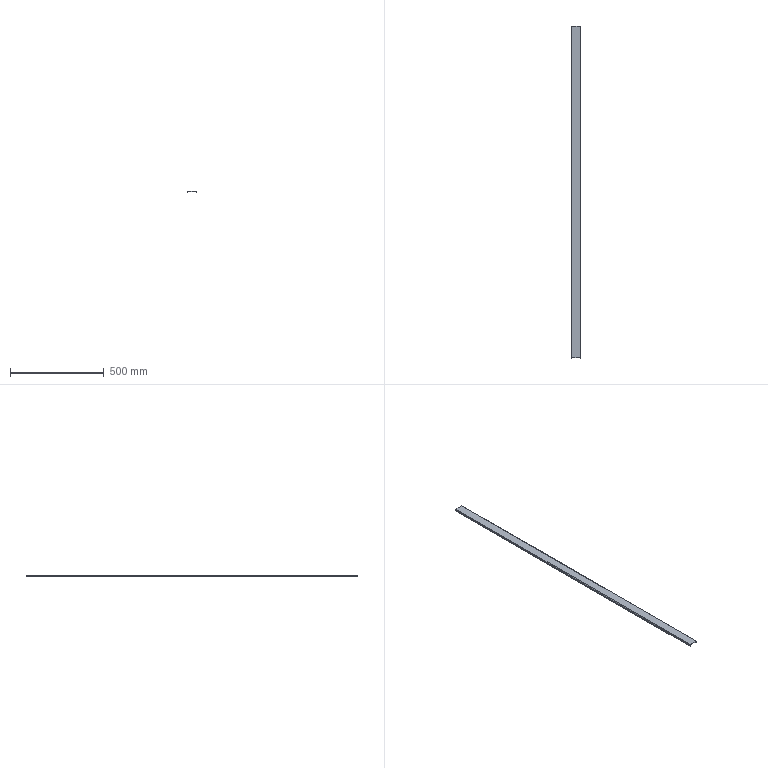Part | SolidWorks | features BaseBody 1 | 1 solid | 22 faces | box 50 x 1772 x 10 mm | volume 281263 mm3 | plane 18 | cylinder 4 | commonest cylinder face diameters 1 x2 6 x2
STEP:
#1=CARTESIAN_POINT('',(-22.5,885.9,-10.));
#2=VERTEX_POINT('',#1);
#3=CARTESIAN_POINT('',(-22.5,-885.9,-10.));
#4=VERTEX_POINT('',#3);
#5=CARTESIAN_POINT('',(-22.5,-885.9,-10.));
#6=DIRECTION('',(0.,-1.,0.));
#7=VECTOR('',#6,1000.);
#8=LINE('',#5,#7);
#9=EDGE_CURVE('',#2,#4,#8,.T.);
#10=ORIENTED_EDGE('',*,*,#9,.T.);
#11=CARTESIAN_POINT('',(-25.,-885.9,-10.));
#12=VERTEX_POINT('',#11);
#13=CARTESIAN_POINT('',(-25.,-885.9,-10.));
#14=DIRECTION('',(1.,0.,0.));
#15=VECTOR('',#14,1000.);
#16=LINE('',#13,#15);
#17=EDGE_CURVE('',#12,#4,#16,.T.);
#18=ORIENTED_EDGE('',*,*,#17,.F.);
#19=CARTESIAN_POINT('',(-25.,885.9,-10.));
#20=VERTEX_POINT('',#19);
#21=CARTESIAN_POINT('',(-25.,0.,-10.));
#22=DIRECTION('',(0.,-1.,0.));
#23=VECTOR('',#22,1000.);
#24=LINE('',#21,#23);
#25=EDGE_CURVE('',#20,#12,#24,.T.);
#26=ORIENTED_EDGE('',*,*,#25,.F.);
#27=CARTESIAN_POINT('',(-25.,885.9,-10.));
#28=DIRECTION('',(1.,0.,0.));
#29=VECTOR('',#28,1000.);
#30=LINE('',#27,#29);
#31=EDGE_CURVE('',#20,#2,#30,.T.);
#32=ORIENTED_EDGE('',*,*,#31,.T.);
#33=EDGE_LOOP('',(#10,#18,#26,#32));
#34=FACE_OUTER_BOUND('',#33,.T.);
#35=CARTESIAN_POINT('',(-25.,-885.9,-10.));
#36=DIRECTION('',(0.,0.,1.));
#37=DIRECTION('',(1.,0.,0.));
#38=AXIS2_PLACEMENT_3D('',#35,#36,#37);
#39=PLANE('',#38);
#40=ADVANCED_FACE('',(#34),#39,.F.);
#41=CARTESIAN_POINT('',(-22.5,885.9,-3.));
#42=VERTEX_POINT('',#41);
#43=CARTESIAN_POINT('',(-22.5,885.9,-10.));
#44=DIRECTION('',(0.,0.,-1.));
#45=VECTOR('',#44,1000.);
#46=LINE('',#43,#45);
#47=EDGE_CURVE('',#42,#2,#46,.T.);
#48=ORIENTED_EDGE('',*,*,#47,.F.);
#49=CARTESIAN_POINT('',(-22.5,-885.9,-3.));
#50=VERTEX_POINT('',#49);
#51=CARTESIAN_POINT('',(-22.5,-885.9,-3.));
#52=DIRECTION('',(0.,1.,0.));
#53=VECTOR('',#52,1000.);
#54=LINE('',#51,#53);
#55=EDGE_CURVE('',#50,#42,#54,.T.);
#56=ORIENTED_EDGE('',*,*,#55,.F.);
#57=CARTESIAN_POINT('',(-22.5,-885.9,-2.5));
#58=DIRECTION('',(0.,0.,1.));
#59=VECTOR('',#58,1000.);
#60=LINE('',#57,#59);
#61=EDGE_CURVE('',#4,#50,#60,.T.);
#62=ORIENTED_EDGE('',*,*,#61,.F.);
#63=ORIENTED_EDGE('',*,*,#9,.F.);
#64=EDGE_LOOP('',(#48,#56,#62,#63));
#65=FACE_OUTER_BOUND('',#64,.T.);
#66=CARTESIAN_POINT('',(-22.5,0.,0.));
#67=DIRECTION('',(1.,0.,0.));
#68=DIRECTION('',(0.,0.,-1.));
#69=AXIS2_PLACEMENT_3D('',#66,#67,#68);
#70=PLANE('',#69);
#71=ADVANCED_FACE('',(#65),#70,.T.);
#72=CARTESIAN_POINT('',(-25.,885.9,-3.));
#73=VERTEX_POINT('',#72);
#74=CARTESIAN_POINT('',(-25.,-885.9,-3.));
#75=VERTEX_POINT('',#74);
#76=CARTESIAN_POINT('',(-25.,-885.9,-3.));
#77=DIRECTION('',(0.,-1.,0.));
#78=VECTOR('',#77,1000.);
#79=LINE('',#76,#78);
#80=EDGE_CURVE('',#73,#75,#79,.T.);
#81=ORIENTED_EDGE('',*,*,#80,.F.);
#82=CARTESIAN_POINT('',(-25.,885.9,0.));
#83=DIRECTION('',(0.,0.,-1.));
#84=VECTOR('',#83,1000.);
#85=LINE('',#82,#84);
#86=EDGE_CURVE('',#73,#20,#85,.T.);
#87=ORIENTED_EDGE('',*,*,#86,.T.);
#88=ORIENTED_EDGE('',*,*,#25,.T.);
#89=CARTESIAN_POINT('',(-25.,-885.9,0.));
#90=DIRECTION('',(0.,0.,1.));
#91=VECTOR('',#90,1000.);
#92=LINE('',#89,#91);
#93=EDGE_CURVE('',#12,#75,#92,.T.);
#94=ORIENTED_EDGE('',*,*,#93,.T.);
#95=EDGE_LOOP('',(#81,#87,#88,#94));
#96=FACE_OUTER_BOUND('',#95,.T.);
#97=CARTESIAN_POINT('',(-25.,0.,0.));
#98=DIRECTION('',(1.,0.,0.));
#99=DIRECTION('',(0.,0.,-1.));
#100=AXIS2_PLACEMENT_3D('',#97,#98,#99);
#101=PLANE('',#100);
#102=ADVANCED_FACE('',(#96),#101,.F.);
#103=CARTESIAN_POINT('',(-25.,-885.9,-3.));
#104=DIRECTION('',(-1.,0.,0.));
#105=VECTOR('',#104,1000.);
#106=LINE('',#103,#105);
#107=EDGE_CURVE('',#50,#75,#106,.T.);
#108=ORIENTED_EDGE('',*,*,#107,.T.);
#109=ORIENTED_EDGE('',*,*,#93,.F.);
#110=ORIENTED_EDGE('',*,*,#17,.T.);
#111=ORIENTED_EDGE('',*,*,#61,.T.);
#112=EDGE_LOOP('',(#108,#109,#110,#111));
#113=FACE_OUTER_BOUND('',#112,.T.);
#114=CARTESIAN_POINT('',(-25.,-885.9,-2.5));
#115=DIRECTION('',(0.,1.,0.));
#116=DIRECTION('',(1.,0.,0.));
#117=AXIS2_PLACEMENT_3D('',#114,#115,#116);
#118=PLANE('',#117);
#119=ADVANCED_FACE('',(#113),#118,.F.);
#120=CARTESIAN_POINT('',(-22.5,885.9,-3.));
#121=DIRECTION('',(-1.,0.,0.));
#122=VECTOR('',#121,1000.);
#123=LINE('',#120,#122);
#124=EDGE_CURVE('',#42,#73,#123,.T.);
#125=ORIENTED_EDGE('',*,*,#124,.F.);
#126=ORIENTED_EDGE('',*,*,#47,.T.);
#127=ORIENTED_EDGE('',*,*,#31,.F.);
#128=ORIENTED_EDGE('',*,*,#86,.F.);
#129=EDGE_LOOP('',(#125,#126,#127,#128));
#130=FACE_OUTER_BOUND('',#129,.T.);
#131=CARTESIAN_POINT('',(-25.,885.9,-10.));
#132=DIRECTION('',(0.,-1.,0.));
#133=DIRECTION('',(0.,0.,-1.));
#134=AXIS2_PLACEMENT_3D('',#131,#132,#133);
#135=PLANE('',#134);
#136=ADVANCED_FACE('',(#130),#135,.F.);
#137=CARTESIAN_POINT('',(-22.,885.9,-2.5));
#138=VERTEX_POINT('',#137);
#139=CARTESIAN_POINT('',(-22.,-885.9,-2.5));
#140=VERTEX_POINT('',#139);
#141=CARTESIAN_POINT('',(-22.,885.9,-2.5));
#142=DIRECTION('',(0.,-1.,0.));
#143=VECTOR('',#142,1000.);
#144=LINE('',#141,#143);
#145=EDGE_CURVE('',#138,#140,#144,.T.);
#146=ORIENTED_EDGE('',*,*,#145,.T.);
#147=CARTESIAN_POINT('',(-22.,-885.9,-3.));
#148=DIRECTION('',(0.,-1.,0.));
#149=DIRECTION('',(0.,0.,1.));
#150=AXIS2_PLACEMENT_3D('',#147,#148,#149);
#151=CIRCLE('',#150,0.5);
#152=EDGE_CURVE('',#140,#50,#151,.T.);
#153=ORIENTED_EDGE('',*,*,#152,.T.);
#154=ORIENTED_EDGE('',*,*,#55,.T.);
#155=CARTESIAN_POINT('',(-22.,885.9,-3.));
#156=DIRECTION('',(0.,1.,0.));
#157=DIRECTION('',(0.,0.,1.));
#158=AXIS2_PLACEMENT_3D('',#155,#156,#157);
#159=CIRCLE('',#158,0.5);
#160=EDGE_CURVE('',#42,#138,#159,.T.);
#161=ORIENTED_EDGE('',*,*,#160,.T.);
#162=EDGE_LOOP('',(#146,#153,#154,#161));
#163=FACE_OUTER_BOUND('',#162,.T.);
#164=CARTESIAN_POINT('',(-22.,885.9,-3.));
#165=DIRECTION('',(0.,1.,0.));
#166=DIRECTION('',(-1.,0.,0.));
#167=AXIS2_PLACEMENT_3D('',#164,#165,#166);
#168=CYLINDRICAL_SURFACE('',#167,0.5);
#169=ADVANCED_FACE('',(#163),#168,.F.);
#170=CARTESIAN_POINT('',(-22.,885.9,0.));
#171=VERTEX_POINT('',#170);
#172=CARTESIAN_POINT('',(-22.,-885.9,0.));
#173=VERTEX_POINT('',#172);
#174=CARTESIAN_POINT('',(-22.,885.9,0.));
#175=DIRECTION('',(0.,-1.,0.));
#176=VECTOR('',#175,1000.);
#177=LINE('',#174,#176);
#178=EDGE_CURVE('',#171,#173,#177,.T.);
#179=ORIENTED_EDGE('',*,*,#178,.F.);
#180=CARTESIAN_POINT('',(-22.,885.9,-3.));
#181=DIRECTION('',(0.,1.,0.));
#182=DIRECTION('',(0.,0.,1.));
#183=AXIS2_PLACEMENT_3D('',#180,#181,#182);
#184=CIRCLE('',#183,3.);
#185=EDGE_CURVE('',#73,#171,#184,.T.);
#186=ORIENTED_EDGE('',*,*,#185,.F.);
#187=ORIENTED_EDGE('',*,*,#80,.T.);
#188=CARTESIAN_POINT('',(-22.,-885.9,-3.));
#189=DIRECTION('',(0.,-1.,0.));
#190=DIRECTION('',(0.,0.,1.));
#191=AXIS2_PLACEMENT_3D('',#188,#189,#190);
#192=CIRCLE('',#191,3.);
#193=EDGE_CURVE('',#173,#75,#192,.T.);
#194=ORIENTED_EDGE('',*,*,#193,.F.);
#195=EDGE_LOOP('',(#179,#186,#187,#194));
#196=FACE_OUTER_BOUND('',#195,.T.);
#197=CARTESIAN_POINT('',(-22.,885.9,-3.));
#198=DIRECTION('',(0.,1.,0.));
#199=DIRECTION('',(-1.,0.,0.));
#200=AXIS2_PLACEMENT_3D('',#197,#198,#199);
#201=CYLINDRICAL_SURFACE('',#200,3.);
#202=ADVANCED_FACE('',(#196),#201,.T.);
#203=ORIENTED_EDGE('',*,*,#160,.F.);
#204=ORIENTED_EDGE('',*,*,#124,.T.);
#205=ORIENTED_EDGE('',*,*,#185,.T.);
#206=CARTESIAN_POINT('',(-22.,885.9,-2.5));
#207=DIRECTION('',(0.,0.,1.));
#208=VECTOR('',#207,1000.);
#209=LINE('',#206,#208);
#210=EDGE_CURVE('',#138,#171,#209,.T.);
#211=ORIENTED_EDGE('',*,*,#210,.F.);
#212=EDGE_LOOP('',(#203,#204,#205,#211));
#213=FACE_OUTER_BOUND('',#212,.T.);
#214=CARTESIAN_POINT('',(-22.,885.9,-3.));
#215=DIRECTION('',(0.,-1.,0.));
#216=DIRECTION('',(0.,0.,-1.));
#217=AXIS2_PLACEMENT_3D('',#214,#215,#216);
#218=PLANE('',#217);
#219=ADVANCED_FACE('',(#213),#218,.F.);
#220=ORIENTED_EDGE('',*,*,#107,.F.);
#221=ORIENTED_EDGE('',*,*,#152,.F.);
#222=CARTESIAN_POINT('',(-22.,-885.9,-2.5));
#223=DIRECTION('',(0.,0.,1.));
#224=VECTOR('',#223,1000.);
#225=LINE('',#222,#224);
#226=EDGE_CURVE('',#140,#173,#225,.T.);
#227=ORIENTED_EDGE('',*,*,#226,.T.);
#228=ORIENTED_EDGE('',*,*,#193,.T.);
#229=EDGE_LOOP('',(#220,#221,#227,#228));
#230=FACE_OUTER_BOUND('',#229,.T.);
#231=CARTESIAN_POINT('',(-22.,-885.9,-3.));
#232=DIRECTION('',(0.,-1.,0.));
#233=DIRECTION('',(0.,0.,-1.));
#234=AXIS2_PLACEMENT_3D('',#231,#232,#233);
#235=PLANE('',#234);
#236=ADVANCED_FACE('',(#230),#235,.T.);
#237=CARTESIAN_POINT('',(22.5,-885.9,-10.));
#238=VERTEX_POINT('',#237);
#239=CARTESIAN_POINT('',(22.5,885.9,-10.));
#240=VERTEX_POINT('',#239);
#241=CARTESIAN_POINT('',(22.5,885.9,-10.));
#242=DIRECTION('',(0.,1.,0.));
#243=VECTOR('',#242,1000.);
#244=LINE('',#241,#243);
#245=EDGE_CURVE('',#238,#240,#244,.T.);
#246=ORIENTED_EDGE('',*,*,#245,.T.);
#247=CARTESIAN_POINT('',(25.,885.9,-10.));
#248=VERTEX_POINT('',#247);
#249=CARTESIAN_POINT('',(25.,885.9,-10.));
#250=DIRECTION('',(-1.,0.,0.));
#251=VECTOR('',#250,1000.);
#252=LINE('',#249,#251);
#253=EDGE_CURVE('',#248,#240,#252,.T.);
#254=ORIENTED_EDGE('',*,*,#253,.F.);
#255=CARTESIAN_POINT('',(25.,-885.9,-10.));
#256=VERTEX_POINT('',#255);
#257=CARTESIAN_POINT('',(25.,0.,-10.));
#258=DIRECTION('',(0.,1.,0.));
#259=VECTOR('',#258,1000.);
#260=LINE('',#257,#259);
#261=EDGE_CURVE('',#256,#248,#260,.T.);
#262=ORIENTED_EDGE('',*,*,#261,.F.);
#263=CARTESIAN_POINT('',(25.,-885.9,-10.));
#264=DIRECTION('',(-1.,0.,0.));
#265=VECTOR('',#264,1000.);
#266=LINE('',#263,#265);
#267=EDGE_CURVE('',#256,#238,#266,.T.);
#268=ORIENTED_EDGE('',*,*,#267,.T.);
#269=EDGE_LOOP('',(#246,#254,#262,#268));
#270=FACE_OUTER_BOUND('',#269,.T.);
#271=CARTESIAN_POINT('',(25.,885.9,-10.));
#272=DIRECTION('',(0.,0.,1.));
#273=DIRECTION('',(1.,0.,0.));
#274=AXIS2_PLACEMENT_3D('',#271,#272,#273);
#275=PLANE('',#274);
#276=ADVANCED_FACE('',(#270),#275,.F.);
#277=CARTESIAN_POINT('',(22.5,-885.9,-3.));
#278=VERTEX_POINT('',#277);
#279=CARTESIAN_POINT('',(22.5,-885.9,-10.));
#280=DIRECTION('',(0.,0.,-1.));
#281=VECTOR('',#280,1000.);
#282=LINE('',#279,#281);
#283=EDGE_CURVE('',#278,#238,#282,.T.);
#284=ORIENTED_EDGE('',*,*,#283,.F.);
#285=CARTESIAN_POINT('',(22.5,885.9,-3.));
#286=VERTEX_POINT('',#285);
#287=CARTESIAN_POINT('',(22.5,885.9,-3.));
#288=DIRECTION('',(0.,-1.,0.));
#289=VECTOR('',#288,1000.);
#290=LINE('',#287,#289);
#291=EDGE_CURVE('',#286,#278,#290,.T.);
#292=ORIENTED_EDGE('',*,*,#291,.F.);
#293=CARTESIAN_POINT('',(22.5,885.9,-2.5));
#294=DIRECTION('',(0.,0.,1.));
#295=VECTOR('',#294,1000.);
#296=LINE('',#293,#295);
#297=EDGE_CURVE('',#240,#286,#296,.T.);
#298=ORIENTED_EDGE('',*,*,#297,.F.);
#299=ORIENTED_EDGE('',*,*,#245,.F.);
#300=EDGE_LOOP('',(#284,#292,#298,#299));
#301=FACE_OUTER_BOUND('',#300,.T.);
#302=CARTESIAN_POINT('',(22.5,0.,0.));
#303=DIRECTION('',(-1.,0.,0.));
#304=DIRECTION('',(0.,0.,1.));
#305=AXIS2_PLACEMENT_3D('',#302,#303,#304);
#306=PLANE('',#305);
#307=ADVANCED_FACE('',(#301),#306,.T.);
#308=CARTESIAN_POINT('',(25.,-885.9,-3.));
#309=VERTEX_POINT('',#308);
#310=CARTESIAN_POINT('',(25.,885.9,-3.));
#311=VERTEX_POINT('',#310);
#312=CARTESIAN_POINT('',(25.,885.9,-3.));
#313=DIRECTION('',(0.,1.,0.));
#314=VECTOR('',#313,1000.);
#315=LINE('',#312,#314);
#316=EDGE_CURVE('',#309,#311,#315,.T.);
#317=ORIENTED_EDGE('',*,*,#316,.F.);
#318=CARTESIAN_POINT('',(25.,-885.9,0.));
#319=DIRECTION('',(0.,0.,-1.));
#320=VECTOR('',#319,1000.);
#321=LINE('',#318,#320);
#322=EDGE_CURVE('',#309,#256,#321,.T.);
#323=ORIENTED_EDGE('',*,*,#322,.T.);
#324=ORIENTED_EDGE('',*,*,#261,.T.);
#325=CARTESIAN_POINT('',(25.,885.9,0.));
#326=DIRECTION('',(0.,0.,1.));
#327=VECTOR('',#326,1000.);
#328=LINE('',#325,#327);
#329=EDGE_CURVE('',#248,#311,#328,.T.);
#330=ORIENTED_EDGE('',*,*,#329,.T.);
#331=EDGE_LOOP('',(#317,#323,#324,#330));
#332=FACE_OUTER_BOUND('',#331,.T.);
#333=CARTESIAN_POINT('',(25.,0.,0.));
#334=DIRECTION('',(-1.,0.,0.));
#335=DIRECTION('',(0.,0.,1.));
#336=AXIS2_PLACEMENT_3D('',#333,#334,#335);
#337=PLANE('',#336);
#338=ADVANCED_FACE('',(#332),#337,.F.);
#339=CARTESIAN_POINT('',(25.,885.9,-3.));
#340=DIRECTION('',(1.,0.,0.));
#341=VECTOR('',#340,1000.);
#342=LINE('',#339,#341);
#343=EDGE_CURVE('',#286,#311,#342,.T.);
#344=ORIENTED_EDGE('',*,*,#343,.T.);
#345=ORIENTED_EDGE('',*,*,#329,.F.);
#346=ORIENTED_EDGE('',*,*,#253,.T.);
#347=ORIENTED_EDGE('',*,*,#297,.T.);
#348=EDGE_LOOP('',(#344,#345,#346,#347));
#349=FACE_OUTER_BOUND('',#348,.T.);
#350=CARTESIAN_POINT('',(25.,885.9,-2.5));
#351=DIRECTION('',(0.,-1.,0.));
#352=DIRECTION('',(0.,0.,-1.));
#353=AXIS2_PLACEMENT_3D('',#350,#351,#352);
#354=PLANE('',#353);
#355=ADVANCED_FACE('',(#349),#354,.F.);
#356=CARTESIAN_POINT('',(22.5,-885.9,-3.));
#357=DIRECTION('',(1.,0.,0.));
#358=VECTOR('',#357,1000.);
#359=LINE('',#356,#358);
#360=EDGE_CURVE('',#278,#309,#359,.T.);
#361=ORIENTED_EDGE('',*,*,#360,.F.);
#362=ORIENTED_EDGE('',*,*,#283,.T.);
#363=ORIENTED_EDGE('',*,*,#267,.F.);
#364=ORIENTED_EDGE('',*,*,#322,.F.);
#365=EDGE_LOOP('',(#361,#362,#363,#364));
#366=FACE_OUTER_BOUND('',#365,.T.);
#367=CARTESIAN_POINT('',(25.,-885.9,-10.));
#368=DIRECTION('',(0.,1.,0.));
#369=DIRECTION('',(1.,0.,0.));
#370=AXIS2_PLACEMENT_3D('',#367,#368,#369);
#371=PLANE('',#370);
#372=ADVANCED_FACE('',(#366),#371,.F.);
#373=CARTESIAN_POINT('',(22.,-885.9,-2.5));
#374=VERTEX_POINT('',#373);
#375=CARTESIAN_POINT('',(22.,885.9,-2.5));
#376=VERTEX_POINT('',#375);
#377=CARTESIAN_POINT('',(22.,-885.9,-2.5));
#378=DIRECTION('',(0.,1.,0.));
#379=VECTOR('',#378,1000.);
#380=LINE('',#377,#379);
#381=EDGE_CURVE('',#374,#376,#380,.T.);
#382=ORIENTED_EDGE('',*,*,#381,.T.);
#383=CARTESIAN_POINT('',(22.,885.9,-3.));
#384=DIRECTION('',(0.,1.,0.));
#385=DIRECTION('',(0.,0.,-1.));
#386=AXIS2_PLACEMENT_3D('',#383,#384,#385);
#387=CIRCLE('',#386,0.5);
#388=EDGE_CURVE('',#376,#286,#387,.T.);
#389=ORIENTED_EDGE('',*,*,#388,.T.);
#390=ORIENTED_EDGE('',*,*,#291,.T.);
#391=CARTESIAN_POINT('',(22.,-885.9,-3.));
#392=DIRECTION('',(0.,-1.,0.));
#393=DIRECTION('',(0.,0.,-1.));
#394=AXIS2_PLACEMENT_3D('',#391,#392,#393);
#395=CIRCLE('',#394,0.5);
#396=EDGE_CURVE('',#278,#374,#395,.T.);
#397=ORIENTED_EDGE('',*,*,#396,.T.);
#398=EDGE_LOOP('',(#382,#389,#390,#397));
#399=FACE_OUTER_BOUND('',#398,.T.);
#400=CARTESIAN_POINT('',(22.,-885.9,-3.));
#401=DIRECTION('',(0.,-1.,0.));
#402=DIRECTION('',(1.,0.,0.));
#403=AXIS2_PLACEMENT_3D('',#400,#401,#402);
#404=CYLINDRICAL_SURFACE('',#403,0.5);
#405=ADVANCED_FACE('',(#399),#404,.F.);
#406=CARTESIAN_POINT('',(22.,-885.9,0.));
#407=VERTEX_POINT('',#406);
#408=CARTESIAN_POINT('',(22.,885.9,0.));
#409=VERTEX_POINT('',#408);
#410=CARTESIAN_POINT('',(22.,-885.9,0.));
#411=DIRECTION('',(0.,1.,0.));
#412=VECTOR('',#411,1000.);
#413=LINE('',#410,#412);
#414=EDGE_CURVE('',#407,#409,#413,.T.);
#415=ORIENTED_EDGE('',*,*,#414,.F.);
#416=CARTESIAN_POINT('',(22.,-885.9,-3.));
#417=DIRECTION('',(0.,-1.,0.));
#418=DIRECTION('',(0.,0.,-1.));
#419=AXIS2_PLACEMENT_3D('',#416,#417,#418);
#420=CIRCLE('',#419,3.);
#421=EDGE_CURVE('',#309,#407,#420,.T.);
#422=ORIENTED_EDGE('',*,*,#421,.F.);
#423=ORIENTED_EDGE('',*,*,#316,.T.);
#424=CARTESIAN_POINT('',(22.,885.9,-3.));
#425=DIRECTION('',(0.,1.,0.));
#426=DIRECTION('',(0.,0.,-1.));
#427=AXIS2_PLACEMENT_3D('',#424,#425,#426);
#428=CIRCLE('',#427,3.);
#429=EDGE_CURVE('',#409,#311,#428,.T.);
#430=ORIENTED_EDGE('',*,*,#429,.F.);
#431=EDGE_LOOP('',(#415,#422,#423,#430));
#432=FACE_OUTER_BOUND('',#431,.T.);
#433=CARTESIAN_POINT('',(22.,-885.9,-3.));
#434=DIRECTION('',(0.,-1.,0.));
#435=DIRECTION('',(1.,0.,0.));
#436=AXIS2_PLACEMENT_3D('',#433,#434,#435);
#437=CYLINDRICAL_SURFACE('',#436,3.);
#438=ADVANCED_FACE('',(#432),#437,.T.);
#439=ORIENTED_EDGE('',*,*,#396,.F.);
#440=ORIENTED_EDGE('',*,*,#360,.T.);
#441=ORIENTED_EDGE('',*,*,#421,.T.);
#442=CARTESIAN_POINT('',(22.,-885.9,-2.5));
#443=DIRECTION('',(0.,0.,1.));
#444=VECTOR('',#443,1000.);
#445=LINE('',#442,#444);
#446=EDGE_CURVE('',#374,#407,#445,.T.);
#447=ORIENTED_EDGE('',*,*,#446,.F.);
#448=EDGE_LOOP('',(#439,#440,#441,#447));
#449=FACE_OUTER_BOUND('',#448,.T.);
#450=CARTESIAN_POINT('',(22.,-885.9,-3.));
#451=DIRECTION('',(0.,1.,0.));
#452=DIRECTION('',(1.,0.,0.));
#453=AXIS2_PLACEMENT_3D('',#450,#451,#452);
#454=PLANE('',#453);
#455=ADVANCED_FACE('',(#449),#454,.F.);
#456=ORIENTED_EDGE('',*,*,#343,.F.);
#457=ORIENTED_EDGE('',*,*,#388,.F.);
#458=CARTESIAN_POINT('',(22.,885.9,-2.5));
#459=DIRECTION('',(0.,0.,1.));
#460=VECTOR('',#459,1000.);
#461=LINE('',#458,#460);
#462=EDGE_CURVE('',#376,#409,#461,.T.);
#463=ORIENTED_EDGE('',*,*,#462,.T.);
#464=ORIENTED_EDGE('',*,*,#429,.T.);
#465=EDGE_LOOP('',(#456,#457,#463,#464));
#466=FACE_OUTER_BOUND('',#465,.T.);
#467=CARTESIAN_POINT('',(22.,885.9,-3.));
#468=DIRECTION('',(0.,1.,0.));
#469=DIRECTION('',(1.,0.,0.));
#470=AXIS2_PLACEMENT_3D('',#467,#468,#469);
#471=PLANE('',#470);
#472=ADVANCED_FACE('',(#466),#471,.T.);
#473=ORIENTED_EDGE('',*,*,#226,.F.);
#474=CARTESIAN_POINT('',(25.,-885.9,-2.5));
#475=DIRECTION('',(1.,0.,0.));
#476=VECTOR('',#475,1000.);
#477=LINE('',#474,#476);
#478=EDGE_CURVE('',#140,#374,#477,.T.);
#479=ORIENTED_EDGE('',*,*,#478,.T.);
#480=ORIENTED_EDGE('',*,*,#446,.T.);
#481=CARTESIAN_POINT('',(25.,-885.9,0.));
#482=DIRECTION('',(1.,0.,0.));
#483=VECTOR('',#482,1000.);
#484=LINE('',#481,#483);
#485=EDGE_CURVE('',#173,#407,#484,.T.);
#486=ORIENTED_EDGE('',*,*,#485,.F.);
#487=EDGE_LOOP('',(#473,#479,#480,#486));
#488=FACE_OUTER_BOUND('',#487,.T.);
#489=CARTESIAN_POINT('',(25.,-885.9,-2.5));
#490=DIRECTION('',(0.,-1.,0.));
#491=DIRECTION('',(0.,0.,-1.));
#492=AXIS2_PLACEMENT_3D('',#489,#490,#491);
#493=PLANE('',#492);
#494=ADVANCED_FACE('',(#488),#493,.T.);
#495=CARTESIAN_POINT('',(25.,885.9,-2.5));
#496=DIRECTION('',(-1.,0.,0.));
#497=VECTOR('',#496,1000.);
#498=LINE('',#495,#497);
#499=EDGE_CURVE('',#376,#138,#498,.T.);
#500=ORIENTED_EDGE('',*,*,#499,.T.);
#501=ORIENTED_EDGE('',*,*,#210,.T.);
#502=CARTESIAN_POINT('',(25.,885.9,0.));
#503=DIRECTION('',(-1.,0.,0.));
#504=VECTOR('',#503,1000.);
#505=LINE('',#502,#504);
#506=EDGE_CURVE('',#409,#171,#505,.T.);
#507=ORIENTED_EDGE('',*,*,#506,.F.);
#508=ORIENTED_EDGE('',*,*,#462,.F.);
#509=EDGE_LOOP('',(#500,#501,#507,#508));
#510=FACE_OUTER_BOUND('',#509,.T.);
#511=CARTESIAN_POINT('',(25.,885.9,-2.5));
#512=DIRECTION('',(0.,1.,0.));
#513=DIRECTION('',(1.,0.,0.));
#514=AXIS2_PLACEMENT_3D('',#511,#512,#513);
#515=PLANE('',#514);
#516=ADVANCED_FACE('',(#510),#515,.T.);
#517=ORIENTED_EDGE('',*,*,#178,.T.);
#518=ORIENTED_EDGE('',*,*,#485,.T.);
#519=ORIENTED_EDGE('',*,*,#414,.T.);
#520=ORIENTED_EDGE('',*,*,#506,.T.);
#521=EDGE_LOOP('',(#517,#518,#519,#520));
#522=FACE_OUTER_BOUND('',#521,.T.);
#523=CARTESIAN_POINT('',(0.,0.,0.));
#524=DIRECTION('',(0.,0.,-1.));
#525=DIRECTION('',(0.,-1.,0.));
#526=AXIS2_PLACEMENT_3D('',#523,#524,#525);
#527=PLANE('',#526);
#528=ADVANCED_FACE('',(#522),#527,.F.);
#529=ORIENTED_EDGE('',*,*,#478,.F.);
#530=ORIENTED_EDGE('',*,*,#145,.F.);
#531=ORIENTED_EDGE('',*,*,#499,.F.);
#532=ORIENTED_EDGE('',*,*,#381,.F.);
#533=EDGE_LOOP('',(#529,#530,#531,#532));
#534=FACE_OUTER_BOUND('',#533,.T.);
#535=CARTESIAN_POINT('',(0.,0.,-2.5));
#536=DIRECTION('',(0.,0.,-1.));
#537=DIRECTION('',(0.,-1.,0.));
#538=AXIS2_PLACEMENT_3D('',#535,#536,#537);
#539=PLANE('',#538);
#540=ADVANCED_FACE('',(#534),#539,.T.);
#541=CLOSED_SHELL('',(#40,#71,#102,#119,#136,#169,#202,#219,#236,#276,#307,#338,#355,#372,#405,#438,#455,#472,#494,#516,#528,#540));
#542=MANIFOLD_SOLID_BREP('',#541);
#543=CARTESIAN_POINT('',(0.,0.,0.));
#544=DIRECTION('',(0.,0.,1.));
#545=DIRECTION('',(1.,0.,0.));
#546=AXIS2_PLACEMENT_3D('',#543,#544,#545);
#547=(LENGTH_UNIT()NAMED_UNIT(*)SI_UNIT(.MILLI.,.METRE.));
#548=UNCERTAINTY_MEASURE_WITH_UNIT(LENGTH_MEASURE(0.00001),#547,'','');
#549=(NAMED_UNIT(*)PLANE_ANGLE_UNIT()SI_UNIT($,.RADIAN.));
#550=(NAMED_UNIT(*)SI_UNIT($,.STERADIAN.)SOLID_ANGLE_UNIT());
#551=(GEOMETRIC_REPRESENTATION_CONTEXT(3)GLOBAL_UNCERTAINTY_ASSIGNED_CONTEXT((#548))GLOBAL_UNIT_ASSIGNED_CONTEXT((#547,#549,#550))REPRESENTATION_CONTEXT('',''));
#552=ADVANCED_BREP_SHAPE_REPRESENTATION('',(#542,#546),#551);